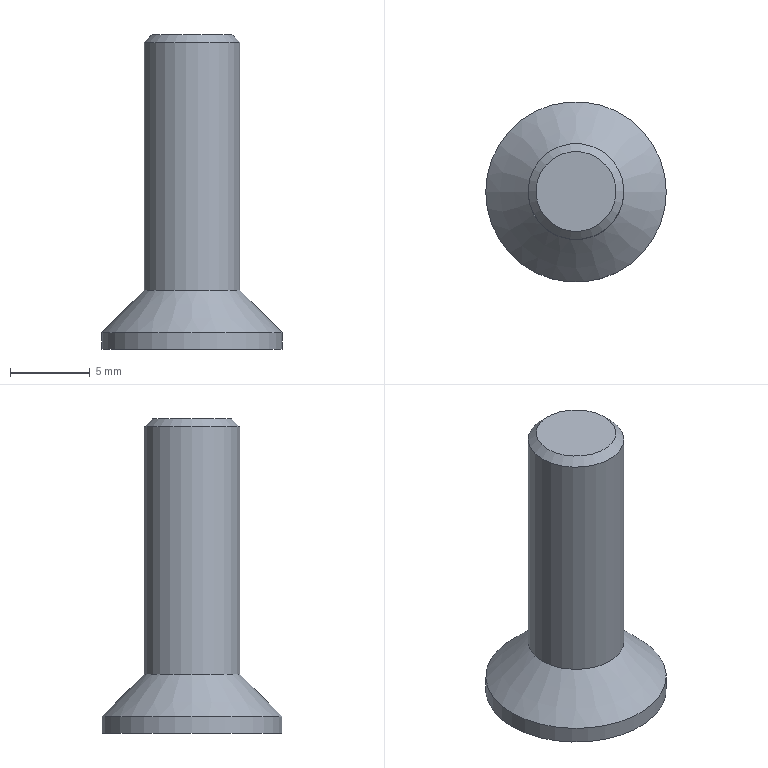Part | STEP file | solid 7 | 1 solid | 13 faces | box 11.3 x 11.3 x 19.7 mm | volume 685.582 mm3 | plane 9 | cylinder 2 | cone 2 | commonest cylinder face diameters 6 x1 11.3 x1